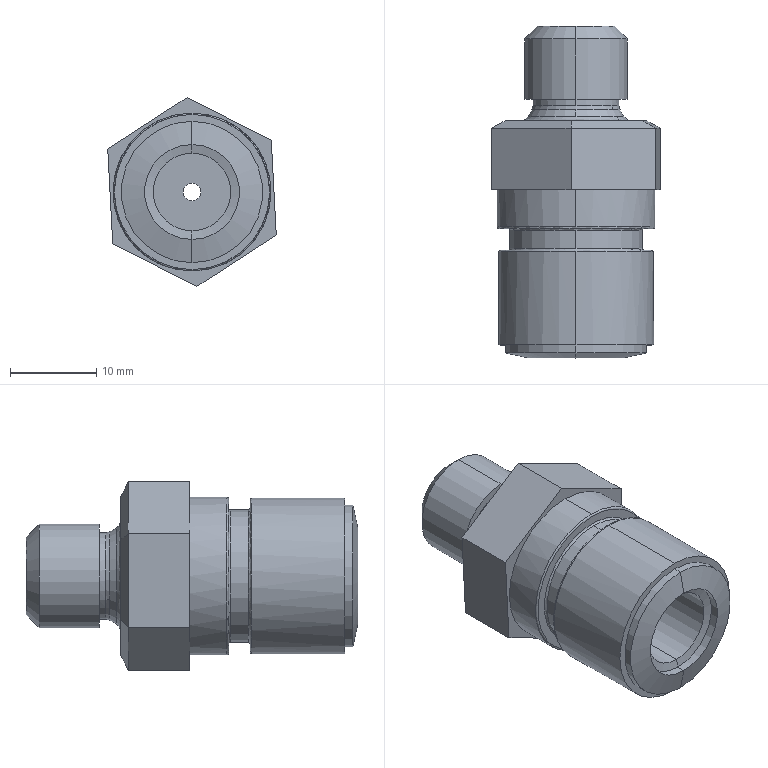Part | SolidWorks | features BaseBody 1 | 1 solid | 60 faces | box 19.551 x 38.5 x 21.909 mm | volume 6617 mm3 | plane 20 | cylinder 18 | spline 12 | cone 10 | commonest cylinder face diameters 2 x2 9 x2 10 x2 11 x2 12 x2 15.4 x2